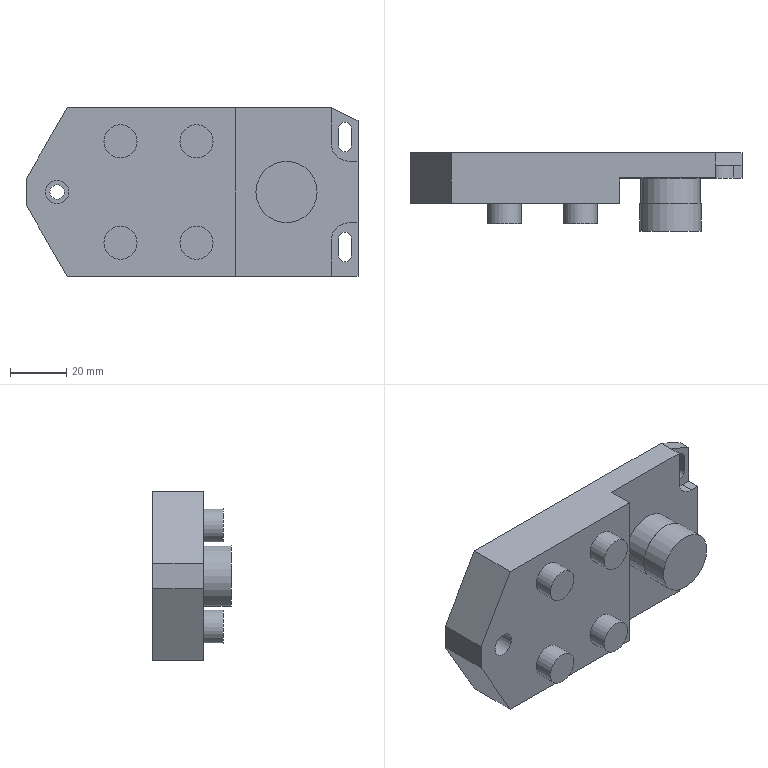Part | STEP file | 1_id718_x_t | 1 solid | 42 faces | box 118 x 27.94 x 59.944 mm | volume 104639 mm3 | plane 28 | cylinder 14 | commonest cylinder face diameters 4.572 x4 11.794 x4 12.7 x2 5.159 x1 8.334 x1 21 x1